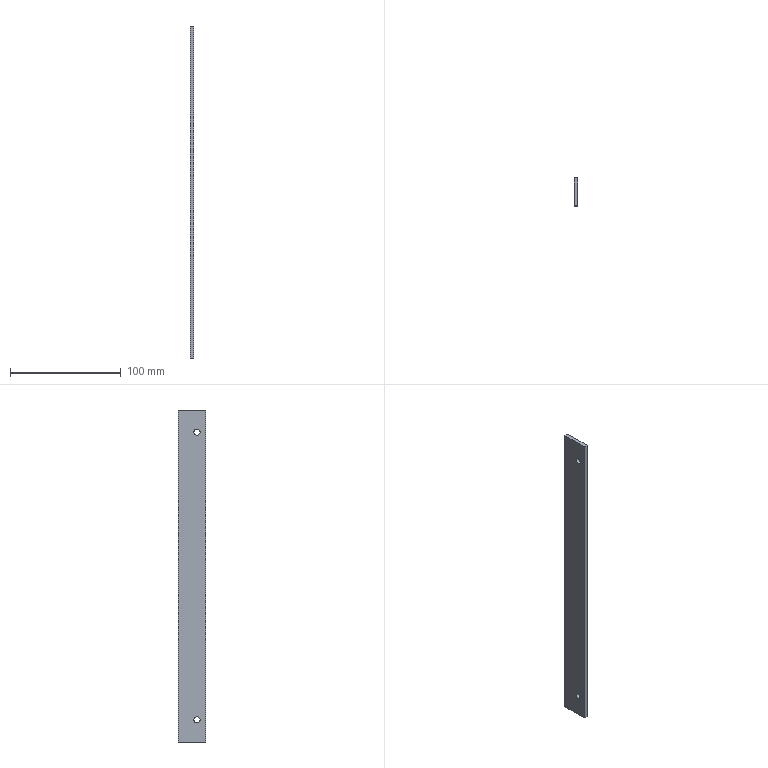Part | STEP file | B1-034 | 1 solid | 10 faces | box 3.5 x 25 x 300 mm | volume 26084 mm3 | plane 6 | cylinder 4 | commonest cylinder face diameters 5.5 x4
STEP:
#1=CARTESIAN_POINT('',(0.,0.,0.));
#2=DIRECTION('',(0.,0.,1.));
#3=DIRECTION('',(1.,0.,0.));
#4=AXIS2_PLACEMENT_3D('',#1,#2,#3);
#5=CARTESIAN_POINT('',(3.5,-4.5,-127.25));
#6=VERTEX_POINT('',#5);
#7=CARTESIAN_POINT('',(0.,-4.5,-127.25));
#8=VERTEX_POINT('',#7);
#9=CARTESIAN_POINT('',(3.5,-4.5,-127.25));
#10=DIRECTION('',(-1.,0.,0.));
#11=VECTOR('',#10,1.);
#12=LINE('',#9,#11);
#13=CARTESIAN_POINT('',(3.5,-4.5,-130.));
#14=DIRECTION('',(-1.,0.,0.));
#15=DIRECTION('',(0.,0.,1.));
#16=AXIS2_PLACEMENT_3D('',#13,#14,#15);
#17=CYLINDRICAL_SURFACE('',#16,2.75);
#18=CARTESIAN_POINT('',(6.283,0.));
#19=DIRECTION('',(0.,1.));
#20=VECTOR('',#19,1.);
#21=LINE('',#18,#20);
#22=(GEOMETRIC_REPRESENTATION_CONTEXT(2)PARAMETRIC_REPRESENTATION_CONTEXT()REPRESENTATION_CONTEXT('',''));
#23=DEFINITIONAL_REPRESENTATION('',(#21),#22);
#24=PCURVE('',#17,#23);
#25=CARTESIAN_POINT('',(3.5,-4.5,-130.));
#26=DIRECTION('',(-1.,0.,0.));
#27=DIRECTION('',(0.,0.,1.));
#28=AXIS2_PLACEMENT_3D('',#25,#26,#27);
#29=CYLINDRICAL_SURFACE('',#28,2.75);
#30=CARTESIAN_POINT('',(0.,0.));
#31=DIRECTION('',(0.,1.));
#32=VECTOR('',#31,1.);
#33=LINE('',#30,#32);
#34=(GEOMETRIC_REPRESENTATION_CONTEXT(2)PARAMETRIC_REPRESENTATION_CONTEXT()REPRESENTATION_CONTEXT('',''));
#35=DEFINITIONAL_REPRESENTATION('',(#33),#34);
#36=PCURVE('',#29,#35);
#37=SURFACE_CURVE('',#12,(#24,#36),.PCURVE_S1.);
#38=EDGE_CURVE('',#6,#8,#37,.T.);
#39=ORIENTED_EDGE('',*,*,#38,.T.);
#40=CARTESIAN_POINT('',(0.,-4.5,-132.75));
#41=VERTEX_POINT('',#40);
#42=CARTESIAN_POINT('',(0.,-4.5,-130.));
#43=DIRECTION('',(1.,0.,0.));
#44=DIRECTION('',(0.,0.,-1.));
#45=AXIS2_PLACEMENT_3D('',#42,#43,#44);
#46=CIRCLE('',#45,2.75);
#47=CARTESIAN_POINT('',(9.425,3.5));
#48=DIRECTION('',(-1.,0.));
#49=VECTOR('',#48,1.);
#50=LINE('',#47,#49);
#51=(GEOMETRIC_REPRESENTATION_CONTEXT(2)PARAMETRIC_REPRESENTATION_CONTEXT()REPRESENTATION_CONTEXT('',''));
#52=DEFINITIONAL_REPRESENTATION('',(#50),#51);
#53=PCURVE('',#17,#52);
#54=CARTESIAN_POINT('',(0.,0.,0.));
#55=DIRECTION('',(1.,0.,0.));
#56=DIRECTION('',(0.,0.,-1.));
#57=AXIS2_PLACEMENT_3D('',#54,#55,#56);
#58=PLANE('',#57);
#59=CARTESIAN_POINT('',(130.,-4.5));
#60=DIRECTION('',(1.,0.));
#61=AXIS2_PLACEMENT_2D('',#59,#60);
#62=CIRCLE('',#61,2.75);
#63=(GEOMETRIC_REPRESENTATION_CONTEXT(2)PARAMETRIC_REPRESENTATION_CONTEXT()REPRESENTATION_CONTEXT('',''));
#64=DEFINITIONAL_REPRESENTATION('',(#62),#63);
#65=PCURVE('',#58,#64);
#66=SURFACE_CURVE('',#46,(#53,#65),.PCURVE_S1.);
#67=EDGE_CURVE('',#8,#41,#66,.T.);
#68=ORIENTED_EDGE('',*,*,#67,.T.);
#69=CARTESIAN_POINT('',(3.5,-4.5,-132.75));
#70=VERTEX_POINT('',#69);
#71=CARTESIAN_POINT('',(3.5,-4.5,-132.75));
#72=DIRECTION('',(-1.,0.,0.));
#73=VECTOR('',#72,1.);
#74=LINE('',#71,#73);
#75=CARTESIAN_POINT('',(3.142,0.));
#76=DIRECTION('',(0.,1.));
#77=VECTOR('',#76,1.);
#78=LINE('',#75,#77);
#79=(GEOMETRIC_REPRESENTATION_CONTEXT(2)PARAMETRIC_REPRESENTATION_CONTEXT()REPRESENTATION_CONTEXT('',''));
#80=DEFINITIONAL_REPRESENTATION('',(#78),#79);
#81=PCURVE('',#17,#80);
#82=CARTESIAN_POINT('',(3.142,0.));
#83=DIRECTION('',(0.,1.));
#84=VECTOR('',#83,1.);
#85=LINE('',#82,#84);
#86=(GEOMETRIC_REPRESENTATION_CONTEXT(2)PARAMETRIC_REPRESENTATION_CONTEXT()REPRESENTATION_CONTEXT('',''));
#87=DEFINITIONAL_REPRESENTATION('',(#85),#86);
#88=PCURVE('',#29,#87);
#89=SURFACE_CURVE('',#74,(#81,#88),.PCURVE_S1.);
#90=EDGE_CURVE('',#70,#41,#89,.T.);
#91=ORIENTED_EDGE('',*,*,#90,.F.);
#92=CARTESIAN_POINT('',(3.5,-4.5,-130.));
#93=DIRECTION('',(1.,0.,0.));
#94=DIRECTION('',(0.,0.,-1.));
#95=AXIS2_PLACEMENT_3D('',#92,#93,#94);
#96=CIRCLE('',#95,2.75);
#97=CARTESIAN_POINT('',(9.425,0.));
#98=DIRECTION('',(-1.,0.));
#99=VECTOR('',#98,1.);
#100=LINE('',#97,#99);
#101=(GEOMETRIC_REPRESENTATION_CONTEXT(2)PARAMETRIC_REPRESENTATION_CONTEXT()REPRESENTATION_CONTEXT('',''));
#102=DEFINITIONAL_REPRESENTATION('',(#100),#101);
#103=PCURVE('',#17,#102);
#104=CARTESIAN_POINT('',(3.5,0.,0.));
#105=DIRECTION('',(1.,0.,0.));
#106=DIRECTION('',(0.,0.,-1.));
#107=AXIS2_PLACEMENT_3D('',#104,#105,#106);
#108=PLANE('',#107);
#109=CARTESIAN_POINT('',(130.,-4.5));
#110=DIRECTION('',(1.,0.));
#111=AXIS2_PLACEMENT_2D('',#109,#110);
#112=CIRCLE('',#111,2.75);
#113=(GEOMETRIC_REPRESENTATION_CONTEXT(2)PARAMETRIC_REPRESENTATION_CONTEXT()REPRESENTATION_CONTEXT('',''));
#114=DEFINITIONAL_REPRESENTATION('',(#112),#113);
#115=PCURVE('',#108,#114);
#116=SURFACE_CURVE('',#96,(#103,#115),.PCURVE_S1.);
#117=EDGE_CURVE('',#6,#70,#116,.T.);
#118=ORIENTED_EDGE('',*,*,#117,.F.);
#119=EDGE_LOOP('',(#39,#68,#91,#118));
#120=FACE_BOUND('',#119,.F.);
#121=ADVANCED_FACE('',(#120),#17,.F.);
#122=CARTESIAN_POINT('',(3.5,-4.5,132.75));
#123=VERTEX_POINT('',#122);
#124=CARTESIAN_POINT('',(0.,-4.5,132.75));
#125=VERTEX_POINT('',#124);
#126=CARTESIAN_POINT('',(3.5,-4.5,132.75));
#127=DIRECTION('',(-1.,0.,0.));
#128=VECTOR('',#127,1.);
#129=LINE('',#126,#128);
#130=CARTESIAN_POINT('',(3.5,-4.5,130.));
#131=DIRECTION('',(-1.,0.,0.));
#132=DIRECTION('',(0.,0.,1.));
#133=AXIS2_PLACEMENT_3D('',#130,#131,#132);
#134=CYLINDRICAL_SURFACE('',#133,2.75);
#135=CARTESIAN_POINT('',(6.283,0.));
#136=DIRECTION('',(0.,1.));
#137=VECTOR('',#136,1.);
#138=LINE('',#135,#137);
#139=(GEOMETRIC_REPRESENTATION_CONTEXT(2)PARAMETRIC_REPRESENTATION_CONTEXT()REPRESENTATION_CONTEXT('',''));
#140=DEFINITIONAL_REPRESENTATION('',(#138),#139);
#141=PCURVE('',#134,#140);
#142=CARTESIAN_POINT('',(3.5,-4.5,130.));
#143=DIRECTION('',(-1.,0.,0.));
#144=DIRECTION('',(0.,0.,1.));
#145=AXIS2_PLACEMENT_3D('',#142,#143,#144);
#146=CYLINDRICAL_SURFACE('',#145,2.75);
#147=CARTESIAN_POINT('',(0.,0.));
#148=DIRECTION('',(0.,1.));
#149=VECTOR('',#148,1.);
#150=LINE('',#147,#149);
#151=(GEOMETRIC_REPRESENTATION_CONTEXT(2)PARAMETRIC_REPRESENTATION_CONTEXT()REPRESENTATION_CONTEXT('',''));
#152=DEFINITIONAL_REPRESENTATION('',(#150),#151);
#153=PCURVE('',#146,#152);
#154=SURFACE_CURVE('',#129,(#141,#153),.PCURVE_S1.);
#155=EDGE_CURVE('',#123,#125,#154,.T.);
#156=ORIENTED_EDGE('',*,*,#155,.T.);
#157=CARTESIAN_POINT('',(0.,-4.5,127.25));
#158=VERTEX_POINT('',#157);
#159=CARTESIAN_POINT('',(0.,-4.5,130.));
#160=DIRECTION('',(1.,0.,0.));
#161=DIRECTION('',(0.,0.,-1.));
#162=AXIS2_PLACEMENT_3D('',#159,#160,#161);
#163=CIRCLE('',#162,2.75);
#164=CARTESIAN_POINT('',(9.425,3.5));
#165=DIRECTION('',(-1.,0.));
#166=VECTOR('',#165,1.);
#167=LINE('',#164,#166);
#168=(GEOMETRIC_REPRESENTATION_CONTEXT(2)PARAMETRIC_REPRESENTATION_CONTEXT()REPRESENTATION_CONTEXT('',''));
#169=DEFINITIONAL_REPRESENTATION('',(#167),#168);
#170=PCURVE('',#134,#169);
#171=CARTESIAN_POINT('',(-130.,-4.5));
#172=DIRECTION('',(1.,0.));
#173=AXIS2_PLACEMENT_2D('',#171,#172);
#174=CIRCLE('',#173,2.75);
#175=(GEOMETRIC_REPRESENTATION_CONTEXT(2)PARAMETRIC_REPRESENTATION_CONTEXT()REPRESENTATION_CONTEXT('',''));
#176=DEFINITIONAL_REPRESENTATION('',(#174),#175);
#177=PCURVE('',#58,#176);
#178=SURFACE_CURVE('',#163,(#170,#177),.PCURVE_S1.);
#179=EDGE_CURVE('',#125,#158,#178,.T.);
#180=ORIENTED_EDGE('',*,*,#179,.T.);
#181=CARTESIAN_POINT('',(3.5,-4.5,127.25));
#182=VERTEX_POINT('',#181);
#183=CARTESIAN_POINT('',(3.5,-4.5,127.25));
#184=DIRECTION('',(-1.,0.,0.));
#185=VECTOR('',#184,1.);
#186=LINE('',#183,#185);
#187=CARTESIAN_POINT('',(3.142,0.));
#188=DIRECTION('',(0.,1.));
#189=VECTOR('',#188,1.);
#190=LINE('',#187,#189);
#191=(GEOMETRIC_REPRESENTATION_CONTEXT(2)PARAMETRIC_REPRESENTATION_CONTEXT()REPRESENTATION_CONTEXT('',''));
#192=DEFINITIONAL_REPRESENTATION('',(#190),#191);
#193=PCURVE('',#134,#192);
#194=CARTESIAN_POINT('',(3.142,0.));
#195=DIRECTION('',(0.,1.));
#196=VECTOR('',#195,1.);
#197=LINE('',#194,#196);
#198=(GEOMETRIC_REPRESENTATION_CONTEXT(2)PARAMETRIC_REPRESENTATION_CONTEXT()REPRESENTATION_CONTEXT('',''));
#199=DEFINITIONAL_REPRESENTATION('',(#197),#198);
#200=PCURVE('',#146,#199);
#201=SURFACE_CURVE('',#186,(#193,#200),.PCURVE_S1.);
#202=EDGE_CURVE('',#182,#158,#201,.T.);
#203=ORIENTED_EDGE('',*,*,#202,.F.);
#204=CARTESIAN_POINT('',(3.5,-4.5,130.));
#205=DIRECTION('',(1.,0.,0.));
#206=DIRECTION('',(0.,0.,-1.));
#207=AXIS2_PLACEMENT_3D('',#204,#205,#206);
#208=CIRCLE('',#207,2.75);
#209=CARTESIAN_POINT('',(9.425,0.));
#210=DIRECTION('',(-1.,0.));
#211=VECTOR('',#210,1.);
#212=LINE('',#209,#211);
#213=(GEOMETRIC_REPRESENTATION_CONTEXT(2)PARAMETRIC_REPRESENTATION_CONTEXT()REPRESENTATION_CONTEXT('',''));
#214=DEFINITIONAL_REPRESENTATION('',(#212),#213);
#215=PCURVE('',#134,#214);
#216=CARTESIAN_POINT('',(-130.,-4.5));
#217=DIRECTION('',(1.,0.));
#218=AXIS2_PLACEMENT_2D('',#216,#217);
#219=CIRCLE('',#218,2.75);
#220=(GEOMETRIC_REPRESENTATION_CONTEXT(2)PARAMETRIC_REPRESENTATION_CONTEXT()REPRESENTATION_CONTEXT('',''));
#221=DEFINITIONAL_REPRESENTATION('',(#219),#220);
#222=PCURVE('',#108,#221);
#223=SURFACE_CURVE('',#208,(#215,#222),.PCURVE_S1.);
#224=EDGE_CURVE('',#123,#182,#223,.T.);
#225=ORIENTED_EDGE('',*,*,#224,.F.);
#226=EDGE_LOOP('',(#156,#180,#203,#225));
#227=FACE_BOUND('',#226,.F.);
#228=ADVANCED_FACE('',(#227),#134,.F.);
#229=ORIENTED_EDGE('',*,*,#224,.F.);
#230=CARTESIAN_POINT('',(3.5,-4.5,130.));
#231=DIRECTION('',(1.,0.,0.));
#232=DIRECTION('',(0.,0.,-1.));
#233=AXIS2_PLACEMENT_3D('',#230,#231,#232);
#234=CIRCLE('',#233,2.75);
#235=CARTESIAN_POINT('',(-130.,-4.5));
#236=DIRECTION('',(1.,0.));
#237=AXIS2_PLACEMENT_2D('',#235,#236);
#238=CIRCLE('',#237,2.75);
#239=(GEOMETRIC_REPRESENTATION_CONTEXT(2)PARAMETRIC_REPRESENTATION_CONTEXT()REPRESENTATION_CONTEXT('',''));
#240=DEFINITIONAL_REPRESENTATION('',(#238),#239);
#241=PCURVE('',#108,#240);
#242=CARTESIAN_POINT('',(3.142,0.));
#243=DIRECTION('',(-1.,0.));
#244=VECTOR('',#243,1.);
#245=LINE('',#242,#244);
#246=(GEOMETRIC_REPRESENTATION_CONTEXT(2)PARAMETRIC_REPRESENTATION_CONTEXT()REPRESENTATION_CONTEXT('',''));
#247=DEFINITIONAL_REPRESENTATION('',(#245),#246);
#248=PCURVE('',#146,#247);
#249=SURFACE_CURVE('',#234,(#241,#248),.PCURVE_S1.);
#250=EDGE_CURVE('',#182,#123,#249,.T.);
#251=ORIENTED_EDGE('',*,*,#250,.F.);
#252=EDGE_LOOP('',(#229,#251));
#253=FACE_BOUND('',#252,.T.);
#254=CARTESIAN_POINT('',(3.5,-12.5,-150.));
#255=VERTEX_POINT('',#254);
#256=CARTESIAN_POINT('',(3.5,12.5,-150.));
#257=VERTEX_POINT('',#256);
#258=CARTESIAN_POINT('',(3.5,12.5,-150.));
#259=DIRECTION('',(0.,1.,0.));
#260=VECTOR('',#259,1.);
#261=LINE('',#258,#260);
#262=CARTESIAN_POINT('',(150.,12.5));
#263=DIRECTION('',(0.,1.));
#264=VECTOR('',#263,1.);
#265=LINE('',#262,#264);
#266=(GEOMETRIC_REPRESENTATION_CONTEXT(2)PARAMETRIC_REPRESENTATION_CONTEXT()REPRESENTATION_CONTEXT('',''));
#267=DEFINITIONAL_REPRESENTATION('',(#265),#266);
#268=PCURVE('',#108,#267);
#269=CARTESIAN_POINT('',(3.5,12.5,-150.));
#270=DIRECTION('',(0.,0.,1.));
#271=DIRECTION('',(1.,0.,0.));
#272=AXIS2_PLACEMENT_3D('',#269,#270,#271);
#273=PLANE('',#272);
#274=CARTESIAN_POINT('',(0.,0.));
#275=DIRECTION('',(0.,1.));
#276=VECTOR('',#275,1.);
#277=LINE('',#274,#276);
#278=(GEOMETRIC_REPRESENTATION_CONTEXT(2)PARAMETRIC_REPRESENTATION_CONTEXT()REPRESENTATION_CONTEXT('',''));
#279=DEFINITIONAL_REPRESENTATION('',(#277),#278);
#280=PCURVE('',#273,#279);
#281=SURFACE_CURVE('',#261,(#268,#280),.PCURVE_S1.);
#282=EDGE_CURVE('',#255,#257,#281,.T.);
#283=ORIENTED_EDGE('',*,*,#282,.T.);
#284=CARTESIAN_POINT('',(3.5,12.5,150.));
#285=VERTEX_POINT('',#284);
#286=CARTESIAN_POINT('',(3.5,12.5,150.));
#287=DIRECTION('',(0.,0.,1.));
#288=VECTOR('',#287,1.);
#289=LINE('',#286,#288);
#290=CARTESIAN_POINT('',(-150.,12.5));
#291=DIRECTION('',(-1.,0.));
#292=VECTOR('',#291,1.);
#293=LINE('',#290,#292);
#294=(GEOMETRIC_REPRESENTATION_CONTEXT(2)PARAMETRIC_REPRESENTATION_CONTEXT()REPRESENTATION_CONTEXT('',''));
#295=DEFINITIONAL_REPRESENTATION('',(#293),#294);
#296=PCURVE('',#108,#295);
#297=CARTESIAN_POINT('',(3.5,12.5,150.));
#298=DIRECTION('',(0.,-1.,0.));
#299=DIRECTION('',(0.,0.,-1.));
#300=AXIS2_PLACEMENT_3D('',#297,#298,#299);
#301=PLANE('',#300);
#302=CARTESIAN_POINT('',(0.,0.));
#303=DIRECTION('',(-1.,0.));
#304=VECTOR('',#303,1.);
#305=LINE('',#302,#304);
#306=(GEOMETRIC_REPRESENTATION_CONTEXT(2)PARAMETRIC_REPRESENTATION_CONTEXT()REPRESENTATION_CONTEXT('',''));
#307=DEFINITIONAL_REPRESENTATION('',(#305),#306);
#308=PCURVE('',#301,#307);
#309=SURFACE_CURVE('',#289,(#296,#308),.PCURVE_S1.);
#310=EDGE_CURVE('',#257,#285,#309,.T.);
#311=ORIENTED_EDGE('',*,*,#310,.T.);
#312=CARTESIAN_POINT('',(3.5,-12.5,150.));
#313=VERTEX_POINT('',#312);
#314=CARTESIAN_POINT('',(3.5,12.5,150.));
#315=DIRECTION('',(0.,-1.,0.));
#316=VECTOR('',#315,1.);
#317=LINE('',#314,#316);
#318=CARTESIAN_POINT('',(-150.,12.5));
#319=DIRECTION('',(0.,-1.));
#320=VECTOR('',#319,1.);
#321=LINE('',#318,#320);
#322=(GEOMETRIC_REPRESENTATION_CONTEXT(2)PARAMETRIC_REPRESENTATION_CONTEXT()REPRESENTATION_CONTEXT('',''));
#323=DEFINITIONAL_REPRESENTATION('',(#321),#322);
#324=PCURVE('',#108,#323);
#325=CARTESIAN_POINT('',(3.5,12.5,150.));
#326=DIRECTION('',(0.,0.,-1.));
#327=DIRECTION('',(-1.,0.,0.));
#328=AXIS2_PLACEMENT_3D('',#325,#326,#327);
#329=PLANE('',#328);
#330=CARTESIAN_POINT('',(0.,0.));
#331=DIRECTION('',(0.,-1.));
#332=VECTOR('',#331,1.);
#333=LINE('',#330,#332);
#334=(GEOMETRIC_REPRESENTATION_CONTEXT(2)PARAMETRIC_REPRESENTATION_CONTEXT()REPRESENTATION_CONTEXT('',''));
#335=DEFINITIONAL_REPRESENTATION('',(#333),#334);
#336=PCURVE('',#329,#335);
#337=SURFACE_CURVE('',#317,(#324,#336),.PCURVE_S1.);
#338=EDGE_CURVE('',#285,#313,#337,.T.);
#339=ORIENTED_EDGE('',*,*,#338,.T.);
#340=CARTESIAN_POINT('',(3.5,-12.5,150.));
#341=DIRECTION('',(0.,0.,-1.));
#342=VECTOR('',#341,1.);
#343=LINE('',#340,#342);
#344=CARTESIAN_POINT('',(-150.,-12.5));
#345=DIRECTION('',(1.,0.));
#346=VECTOR('',#345,1.);
#347=LINE('',#344,#346);
#348=(GEOMETRIC_REPRESENTATION_CONTEXT(2)PARAMETRIC_REPRESENTATION_CONTEXT()REPRESENTATION_CONTEXT('',''));
#349=DEFINITIONAL_REPRESENTATION('',(#347),#348);
#350=PCURVE('',#108,#349);
#351=CARTESIAN_POINT('',(3.5,-12.5,150.));
#352=DIRECTION('',(0.,1.,0.));
#353=DIRECTION('',(0.,0.,1.));
#354=AXIS2_PLACEMENT_3D('',#351,#352,#353);
#355=PLANE('',#354);
#356=CARTESIAN_POINT('',(0.,0.));
#357=DIRECTION('',(-1.,0.));
#358=VECTOR('',#357,1.);
#359=LINE('',#356,#358);
#360=(GEOMETRIC_REPRESENTATION_CONTEXT(2)PARAMETRIC_REPRESENTATION_CONTEXT()REPRESENTATION_CONTEXT('',''));
#361=DEFINITIONAL_REPRESENTATION('',(#359),#360);
#362=PCURVE('',#355,#361);
#363=SURFACE_CURVE('',#343,(#350,#362),.PCURVE_S1.);
#364=EDGE_CURVE('',#313,#255,#363,.T.);
#365=ORIENTED_EDGE('',*,*,#364,.T.);
#366=EDGE_LOOP('',(#283,#311,#339,#365));
#367=FACE_BOUND('',#366,.T.);
#368=ORIENTED_EDGE('',*,*,#117,.F.);
#369=CARTESIAN_POINT('',(3.5,-4.5,-130.));
#370=DIRECTION('',(1.,0.,0.));
#371=DIRECTION('',(0.,0.,-1.));
#372=AXIS2_PLACEMENT_3D('',#369,#370,#371);
#373=CIRCLE('',#372,2.75);
#374=CARTESIAN_POINT('',(130.,-4.5));
#375=DIRECTION('',(1.,0.));
#376=AXIS2_PLACEMENT_2D('',#374,#375);
#377=CIRCLE('',#376,2.75);
#378=(GEOMETRIC_REPRESENTATION_CONTEXT(2)PARAMETRIC_REPRESENTATION_CONTEXT()REPRESENTATION_CONTEXT('',''));
#379=DEFINITIONAL_REPRESENTATION('',(#377),#378);
#380=PCURVE('',#108,#379);
#381=CARTESIAN_POINT('',(3.142,0.));
#382=DIRECTION('',(-1.,0.));
#383=VECTOR('',#382,1.);
#384=LINE('',#381,#383);
#385=(GEOMETRIC_REPRESENTATION_CONTEXT(2)PARAMETRIC_REPRESENTATION_CONTEXT()REPRESENTATION_CONTEXT('',''));
#386=DEFINITIONAL_REPRESENTATION('',(#384),#385);
#387=PCURVE('',#29,#386);
#388=SURFACE_CURVE('',#373,(#380,#387),.PCURVE_S1.);
#389=EDGE_CURVE('',#70,#6,#388,.T.);
#390=ORIENTED_EDGE('',*,*,#389,.F.);
#391=EDGE_LOOP('',(#368,#390));
#392=FACE_BOUND('',#391,.T.);
#393=ADVANCED_FACE('',(#253,#367,#392),#108,.T.);
#394=CARTESIAN_POINT('',(0.,-12.5,-150.));
#395=VERTEX_POINT('',#394);
#396=CARTESIAN_POINT('',(0.,12.5,-150.));
#397=VERTEX_POINT('',#396);
#398=CARTESIAN_POINT('',(0.,12.5,-150.));
#399=DIRECTION('',(0.,1.,0.));
#400=VECTOR('',#399,1.);
#401=LINE('',#398,#400);
#402=CARTESIAN_POINT('',(150.,12.5));
#403=DIRECTION('',(0.,1.));
#404=VECTOR('',#403,1.);
#405=LINE('',#402,#404);
#406=(GEOMETRIC_REPRESENTATION_CONTEXT(2)PARAMETRIC_REPRESENTATION_CONTEXT()REPRESENTATION_CONTEXT('',''));
#407=DEFINITIONAL_REPRESENTATION('',(#405),#406);
#408=PCURVE('',#58,#407);
#409=CARTESIAN_POINT('',(-3.5,0.));
#410=DIRECTION('',(0.,1.));
#411=VECTOR('',#410,1.);
#412=LINE('',#409,#411);
#413=(GEOMETRIC_REPRESENTATION_CONTEXT(2)PARAMETRIC_REPRESENTATION_CONTEXT()REPRESENTATION_CONTEXT('',''));
#414=DEFINITIONAL_REPRESENTATION('',(#412),#413);
#415=PCURVE('',#273,#414);
#416=SURFACE_CURVE('',#401,(#408,#415),.PCURVE_S1.);
#417=EDGE_CURVE('',#395,#397,#416,.T.);
#418=ORIENTED_EDGE('',*,*,#417,.F.);
#419=CARTESIAN_POINT('',(0.,-12.5,150.));
#420=VERTEX_POINT('',#419);
#421=CARTESIAN_POINT('',(0.,-12.5,150.));
#422=DIRECTION('',(0.,0.,-1.));
#423=VECTOR('',#422,1.);
#424=LINE('',#421,#423);
#425=CARTESIAN_POINT('',(-150.,-12.5));
#426=DIRECTION('',(1.,0.));
#427=VECTOR('',#426,1.);
#428=LINE('',#425,#427);
#429=(GEOMETRIC_REPRESENTATION_CONTEXT(2)PARAMETRIC_REPRESENTATION_CONTEXT()REPRESENTATION_CONTEXT('',''));
#430=DEFINITIONAL_REPRESENTATION('',(#428),#429);
#431=PCURVE('',#58,#430);
#432=CARTESIAN_POINT('',(0.,-3.5));
#433=DIRECTION('',(-1.,0.));
#434=VECTOR('',#433,1.);
#435=LINE('',#432,#434);
#436=(GEOMETRIC_REPRESENTATION_CONTEXT(2)PARAMETRIC_REPRESENTATION_CONTEXT()REPRESENTATION_CONTEXT('',''));
#437=DEFINITIONAL_REPRESENTATION('',(#435),#436);
#438=PCURVE('',#355,#437);
#439=SURFACE_CURVE('',#424,(#431,#438),.PCURVE_S1.);
#440=EDGE_CURVE('',#420,#395,#439,.T.);
#441=ORIENTED_EDGE('',*,*,#440,.F.);
#442=CARTESIAN_POINT('',(0.,12.5,150.));
#443=VERTEX_POINT('',#442);
#444=CARTESIAN_POINT('',(0.,12.5,150.));
#445=DIRECTION('',(0.,-1.,0.));
#446=VECTOR('',#445,1.);
#447=LINE('',#444,#446);
#448=CARTESIAN_POINT('',(-150.,12.5));
#449=DIRECTION('',(0.,-1.));
#450=VECTOR('',#449,1.);
#451=LINE('',#448,#450);
#452=(GEOMETRIC_REPRESENTATION_CONTEXT(2)PARAMETRIC_REPRESENTATION_CONTEXT()REPRESENTATION_CONTEXT('',''));
#453=DEFINITIONAL_REPRESENTATION('',(#451),#452);
#454=PCURVE('',#58,#453);
#455=CARTESIAN_POINT('',(3.5,0.));
#456=DIRECTION('',(0.,-1.));
#457=VECTOR('',#456,1.);
#458=LINE('',#455,#457);
#459=(GEOMETRIC_REPRESENTATION_CONTEXT(2)PARAMETRIC_REPRESENTATION_CONTEXT()REPRESENTATION_CONTEXT('',''));
#460=DEFINITIONAL_REPRESENTATION('',(#458),#459);
#461=PCURVE('',#329,#460);
#462=SURFACE_CURVE('',#447,(#454,#461),.PCURVE_S1.);
#463=EDGE_CURVE('',#443,#420,#462,.T.);
#464=ORIENTED_EDGE('',*,*,#463,.F.);
#465=CARTESIAN_POINT('',(0.,12.5,150.));
#466=DIRECTION('',(0.,0.,1.));
#467=VECTOR('',#466,1.);
#468=LINE('',#465,#467);
#469=CARTESIAN_POINT('',(-150.,12.5));
#470=DIRECTION('',(-1.,0.));
#471=VECTOR('',#470,1.);
#472=LINE('',#469,#471);
#473=(GEOMETRIC_REPRESENTATION_CONTEXT(2)PARAMETRIC_REPRESENTATION_CONTEXT()REPRESENTATION_CONTEXT('',''));
#474=DEFINITIONAL_REPRESENTATION('',(#472),#473);
#475=PCURVE('',#58,#474);
#476=CARTESIAN_POINT('',(0.,-3.5));
#477=DIRECTION('',(-1.,0.));
#478=VECTOR('',#477,1.);
#479=LINE('',#476,#478);
#480=(GEOMETRIC_REPRESENTATION_CONTEXT(2)PARAMETRIC_REPRESENTATION_CONTEXT()REPRESENTATION_CONTEXT('',''));
#481=DEFINITIONAL_REPRESENTATION('',(#479),#480);
#482=PCURVE('',#301,#481);
#483=SURFACE_CURVE('',#468,(#475,#482),.PCURVE_S1.);
#484=EDGE_CURVE('',#397,#443,#483,.T.);
#485=ORIENTED_EDGE('',*,*,#484,.F.);
#486=EDGE_LOOP('',(#418,#441,#464,#485));
#487=FACE_BOUND('',#486,.T.);
#488=ORIENTED_EDGE('',*,*,#179,.T.);
#489=CARTESIAN_POINT('',(0.,-4.5,130.));
#490=DIRECTION('',(1.,0.,0.));
#491=DIRECTION('',(0.,0.,-1.));
#492=AXIS2_PLACEMENT_3D('',#489,#490,#491);
#493=CIRCLE('',#492,2.75);
#494=CARTESIAN_POINT('',(-130.,-4.5));
#495=DIRECTION('',(1.,0.));
#496=AXIS2_PLACEMENT_2D('',#494,#495);
#497=CIRCLE('',#496,2.75);
#498=(GEOMETRIC_REPRESENTATION_CONTEXT(2)PARAMETRIC_REPRESENTATION_CONTEXT()REPRESENTATION_CONTEXT('',''));
#499=DEFINITIONAL_REPRESENTATION('',(#497),#498);
#500=PCURVE('',#58,#499);
#501=CARTESIAN_POINT('',(3.142,3.5));
#502=DIRECTION('',(-1.,0.));
#503=VECTOR('',#502,1.);
#504=LINE('',#501,#503);
#505=(GEOMETRIC_REPRESENTATION_CONTEXT(2)PARAMETRIC_REPRESENTATION_CONTEXT()REPRESENTATION_CONTEXT('',''));
#506=DEFINITIONAL_REPRESENTATION('',(#504),#505);
#507=PCURVE('',#146,#506);
#508=SURFACE_CURVE('',#493,(#500,#507),.PCURVE_S1.);
#509=EDGE_CURVE('',#158,#125,#508,.T.);
#510=ORIENTED_EDGE('',*,*,#509,.T.);
#511=EDGE_LOOP('',(#488,#510));
#512=FACE_BOUND('',#511,.T.);
#513=ORIENTED_EDGE('',*,*,#67,.T.);
#514=CARTESIAN_POINT('',(0.,-4.5,-130.));
#515=DIRECTION('',(1.,0.,0.));
#516=DIRECTION('',(0.,0.,-1.));
#517=AXIS2_PLACEMENT_3D('',#514,#515,#516);
#518=CIRCLE('',#517,2.75);
#519=CARTESIAN_POINT('',(130.,-4.5));
#520=DIRECTION('',(1.,0.));
#521=AXIS2_PLACEMENT_2D('',#519,#520);
#522=CIRCLE('',#521,2.75);
#523=(GEOMETRIC_REPRESENTATION_CONTEXT(2)PARAMETRIC_REPRESENTATION_CONTEXT()REPRESENTATION_CONTEXT('',''));
#524=DEFINITIONAL_REPRESENTATION('',(#522),#523);
#525=PCURVE('',#58,#524);
#526=CARTESIAN_POINT('',(3.142,3.5));
#527=DIRECTION('',(-1.,0.));
#528=VECTOR('',#527,1.);
#529=LINE('',#526,#528);
#530=(GEOMETRIC_REPRESENTATION_CONTEXT(2)PARAMETRIC_REPRESENTATION_CONTEXT()REPRESENTATION_CONTEXT('',''));
#531=DEFINITIONAL_REPRESENTATION('',(#529),#530);
#532=PCURVE('',#29,#531);
#533=SURFACE_CURVE('',#518,(#525,#532),.PCURVE_S1.);
#534=EDGE_CURVE('',#41,#8,#533,.T.);
#535=ORIENTED_EDGE('',*,*,#534,.T.);
#536=EDGE_LOOP('',(#513,#535));
#537=FACE_BOUND('',#536,.T.);
#538=ADVANCED_FACE('',(#487,#512,#537),#58,.F.);
#539=ORIENTED_EDGE('',*,*,#417,.T.);
#540=CARTESIAN_POINT('',(3.5,12.5,-150.));
#541=DIRECTION('',(-1.,0.,0.));
#542=VECTOR('',#541,1.);
#543=LINE('',#540,#542);
#544=CARTESIAN_POINT('',(0.,0.));
#545=DIRECTION('',(-1.,0.));
#546=VECTOR('',#545,1.);
#547=LINE('',#544,#546);
#548=(GEOMETRIC_REPRESENTATION_CONTEXT(2)PARAMETRIC_REPRESENTATION_CONTEXT()REPRESENTATION_CONTEXT('',''));
#549=DEFINITIONAL_REPRESENTATION('',(#547),#548);
#550=PCURVE('',#273,#549);
#551=CARTESIAN_POINT('',(300.,0.));
#552=DIRECTION('',(0.,-1.));
#553=VECTOR('',#552,1.);
#554=LINE('',#551,#553);
#555=(GEOMETRIC_REPRESENTATION_CONTEXT(2)PARAMETRIC_REPRESENTATION_CONTEXT()REPRESENTATION_CONTEXT('',''));
#556=DEFINITIONAL_REPRESENTATION('',(#554),#555);
#557=PCURVE('',#301,#556);
#558=SURFACE_CURVE('',#543,(#550,#557),.PCURVE_S1.);
#559=EDGE_CURVE('',#257,#397,#558,.T.);
#560=ORIENTED_EDGE('',*,*,#559,.F.);
#561=ORIENTED_EDGE('',*,*,#282,.F.);
#562=CARTESIAN_POINT('',(3.5,-12.5,-150.));
#563=DIRECTION('',(-1.,0.,0.));
#564=VECTOR('',#563,1.);
#565=LINE('',#562,#564);
#566=CARTESIAN_POINT('',(0.,-25.));
#567=DIRECTION('',(-1.,0.));
#568=VECTOR('',#567,1.);
#569=LINE('',#566,#568);
#570=(GEOMETRIC_REPRESENTATION_CONTEXT(2)PARAMETRIC_REPRESENTATION_CONTEXT()REPRESENTATION_CONTEXT('',''));
#571=DEFINITIONAL_REPRESENTATION('',(#569),#570);
#572=PCURVE('',#273,#571);
#573=CARTESIAN_POINT('',(-300.,0.));
#574=DIRECTION('',(0.,-1.));
#575=VECTOR('',#574,1.);
#576=LINE('',#573,#575);
#577=(GEOMETRIC_REPRESENTATION_CONTEXT(2)PARAMETRIC_REPRESENTATION_CONTEXT()REPRESENTATION_CONTEXT('',''));
#578=DEFINITIONAL_REPRESENTATION('',(#576),#577);
#579=PCURVE('',#355,#578);
#580=SURFACE_CURVE('',#565,(#572,#579),.PCURVE_S1.);
#581=EDGE_CURVE('',#255,#395,#580,.T.);
#582=ORIENTED_EDGE('',*,*,#581,.T.);
#583=EDGE_LOOP('',(#539,#560,#561,#582));
#584=FACE_BOUND('',#583,.T.);
#585=ADVANCED_FACE('',(#584),#273,.F.);
#586=ORIENTED_EDGE('',*,*,#484,.T.);
#587=CARTESIAN_POINT('',(3.5,12.5,150.));
#588=DIRECTION('',(-1.,0.,0.));
#589=VECTOR('',#588,1.);
#590=LINE('',#587,#589);
#591=CARTESIAN_POINT('',(0.,0.));
#592=DIRECTION('',(0.,-1.));
#593=VECTOR('',#592,1.);
#594=LINE('',#591,#593);
#595=(GEOMETRIC_REPRESENTATION_CONTEXT(2)PARAMETRIC_REPRESENTATION_CONTEXT()REPRESENTATION_CONTEXT('',''));
#596=DEFINITIONAL_REPRESENTATION('',(#594),#595);
#597=PCURVE('',#301,#596);
#598=CARTESIAN_POINT('',(0.,0.));
#599=DIRECTION('',(1.,0.));
#600=VECTOR('',#599,1.);
#601=LINE('',#598,#600);
#602=(GEOMETRIC_REPRESENTATION_CONTEXT(2)PARAMETRIC_REPRESENTATION_CONTEXT()REPRESENTATION_CONTEXT('',''));
#603=DEFINITIONAL_REPRESENTATION('',(#601),#602);
#604=PCURVE('',#329,#603);
#605=SURFACE_CURVE('',#590,(#597,#604),.PCURVE_S1.);
#606=EDGE_CURVE('',#285,#443,#605,.T.);
#607=ORIENTED_EDGE('',*,*,#606,.F.);
#608=ORIENTED_EDGE('',*,*,#310,.F.);
#609=ORIENTED_EDGE('',*,*,#559,.T.);
#610=EDGE_LOOP('',(#586,#607,#608,#609));
#611=FACE_BOUND('',#610,.T.);
#612=ADVANCED_FACE('',(#611),#301,.F.);
#613=ORIENTED_EDGE('',*,*,#463,.T.);
#614=CARTESIAN_POINT('',(3.5,-12.5,150.));
#615=DIRECTION('',(-1.,0.,0.));
#616=VECTOR('',#615,1.);
#617=LINE('',#614,#616);
#618=CARTESIAN_POINT('',(0.,-25.));
#619=DIRECTION('',(1.,0.));
#620=VECTOR('',#619,1.);
#621=LINE('',#618,#620);
#622=(GEOMETRIC_REPRESENTATION_CONTEXT(2)PARAMETRIC_REPRESENTATION_CONTEXT()REPRESENTATION_CONTEXT('',''));
#623=DEFINITIONAL_REPRESENTATION('',(#621),#622);
#624=PCURVE('',#329,#623);
#625=CARTESIAN_POINT('',(0.,0.));
#626=DIRECTION('',(0.,-1.));
#627=VECTOR('',#626,1.);
#628=LINE('',#625,#627);
#629=(GEOMETRIC_REPRESENTATION_CONTEXT(2)PARAMETRIC_REPRESENTATION_CONTEXT()REPRESENTATION_CONTEXT('',''));
#630=DEFINITIONAL_REPRESENTATION('',(#628),#629);
#631=PCURVE('',#355,#630);
#632=SURFACE_CURVE('',#617,(#624,#631),.PCURVE_S1.);
#633=EDGE_CURVE('',#313,#420,#632,.T.);
#634=ORIENTED_EDGE('',*,*,#633,.F.);
#635=ORIENTED_EDGE('',*,*,#338,.F.);
#636=ORIENTED_EDGE('',*,*,#606,.T.);
#637=EDGE_LOOP('',(#613,#634,#635,#636));
#638=FACE_BOUND('',#637,.T.);
#639=ADVANCED_FACE('',(#638),#329,.F.);
#640=ORIENTED_EDGE('',*,*,#440,.T.);
#641=ORIENTED_EDGE('',*,*,#581,.F.);
#642=ORIENTED_EDGE('',*,*,#364,.F.);
#643=ORIENTED_EDGE('',*,*,#633,.T.);
#644=EDGE_LOOP('',(#640,#641,#642,#643));
#645=FACE_BOUND('',#644,.T.);
#646=ADVANCED_FACE('',(#645),#355,.F.);
#647=ORIENTED_EDGE('',*,*,#509,.T.);
#648=ORIENTED_EDGE('',*,*,#155,.F.);
#649=ORIENTED_EDGE('',*,*,#250,.F.);
#650=ORIENTED_EDGE('',*,*,#202,.T.);
#651=EDGE_LOOP('',(#647,#648,#649,#650));
#652=FACE_BOUND('',#651,.F.);
#653=ADVANCED_FACE('',(#652),#146,.F.);
#654=ORIENTED_EDGE('',*,*,#534,.T.);
#655=ORIENTED_EDGE('',*,*,#38,.F.);
#656=ORIENTED_EDGE('',*,*,#389,.F.);
#657=ORIENTED_EDGE('',*,*,#90,.T.);
#658=EDGE_LOOP('',(#654,#655,#656,#657));
#659=FACE_BOUND('',#658,.F.);
#660=ADVANCED_FACE('',(#659),#29,.F.);
#661=CLOSED_SHELL('',(#121,#228,#393,#538,#585,#612,#639,#646,#653,#660));
#662=MANIFOLD_SOLID_BREP('',#661);
#663=(LENGTH_UNIT()NAMED_UNIT(*)SI_UNIT(.MILLI.,.METRE.));
#664=UNCERTAINTY_MEASURE_WITH_UNIT(LENGTH_MEASURE(0.0000001),#663,'','');
#665=(NAMED_UNIT(*)PLANE_ANGLE_UNIT()SI_UNIT($,.RADIAN.));
#666=(NAMED_UNIT(*)SI_UNIT($,.STERADIAN.)SOLID_ANGLE_UNIT());
#667=(GEOMETRIC_REPRESENTATION_CONTEXT(3)GLOBAL_UNCERTAINTY_ASSIGNED_CONTEXT((#664))GLOBAL_UNIT_ASSIGNED_CONTEXT((#663,#665,#666))REPRESENTATION_CONTEXT('',''));
#668=ADVANCED_BREP_SHAPE_REPRESENTATION('',(#4,#662),#667);